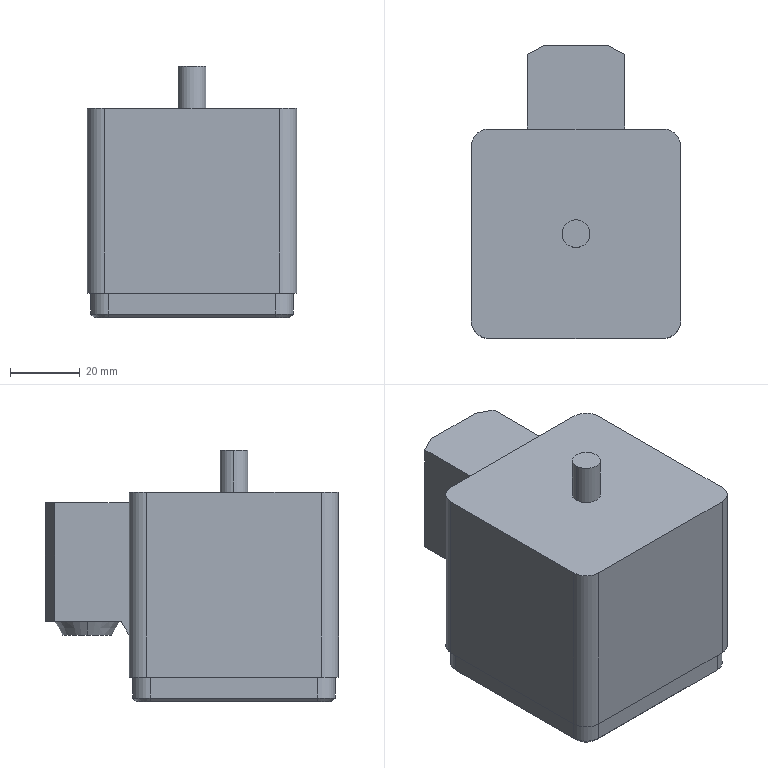Part | SolidWorks | features ICE 5, Fillet 2, Chamfer 1, Extrusion 1 | 1 solid | 41 faces | box 60 x 84 x 72 mm | volume 236948 mm3 | plane 25 | cylinder 10 | cone 6 | commonest cylinder face diameters 10 x8 8 x2
STEP:
#1=CARTESIAN_POINT('',(7.084,42.,19.));
#2=VERTEX_POINT('',#1);
#3=CARTESIAN_POINT('',(-7.084,42.,19.));
#4=VERTEX_POINT('',#3);
#5=CARTESIAN_POINT('',(0.,42.,19.));
#6=DIRECTION('',(0.,0.,-1.));
#7=DIRECTION('',(-1.,0.,0.));
#8=AXIS2_PLACEMENT_3D('',#5,#6,#7);
#9=CIRCLE('',#8,7.084);
#10=EDGE_CURVE('',#2,#4,#9,.T.);
#11=ORIENTED_EDGE('',*,*,#10,.F.);
#12=CARTESIAN_POINT('',(9.393,42.,23.));
#13=VERTEX_POINT('',#12);
#14=CARTESIAN_POINT('',(7.084,42.,19.));
#15=DIRECTION('',(0.5,0.,0.866));
#16=VECTOR('',#15,1000.);
#17=LINE('',#14,#16);
#18=EDGE_CURVE('',#2,#13,#17,.T.);
#19=ORIENTED_EDGE('',*,*,#18,.T.);
#20=CARTESIAN_POINT('',(-9.393,42.,23.));
#21=VERTEX_POINT('',#20);
#22=CARTESIAN_POINT('',(0.,42.,23.));
#23=DIRECTION('',(0.,0.,-1.));
#24=DIRECTION('',(-1.,0.,0.));
#25=AXIS2_PLACEMENT_3D('',#22,#23,#24);
#26=CIRCLE('',#25,9.393);
#27=EDGE_CURVE('',#13,#21,#26,.T.);
#28=ORIENTED_EDGE('',*,*,#27,.T.);
#29=CARTESIAN_POINT('',(-7.084,42.,19.));
#30=DIRECTION('',(-0.5,0.,0.866));
#31=VECTOR('',#30,1000.);
#32=LINE('',#29,#31);
#33=EDGE_CURVE('',#4,#21,#32,.T.);
#34=ORIENTED_EDGE('',*,*,#33,.F.);
#35=EDGE_LOOP('',(#11,#19,#28,#34));
#36=FACE_OUTER_BOUND('',#35,.T.);
#37=CARTESIAN_POINT('',(0.,42.,19.));
#38=DIRECTION('',(0.,0.,1.));
#39=DIRECTION('',(-1.,0.,0.));
#40=AXIS2_PLACEMENT_3D('',#37,#38,#39);
#41=CONICAL_SURFACE('',#40,7.084,0.5236);
#42=ADVANCED_FACE('',(#36),#41,.T.);
#43=CARTESIAN_POINT('',(4.,0.,72.));
#44=VERTEX_POINT('',#43);
#45=CARTESIAN_POINT('',(-4.,0.,72.));
#46=VERTEX_POINT('',#45);
#47=CARTESIAN_POINT('',(0.,0.,72.));
#48=DIRECTION('',(0.,0.,1.));
#49=DIRECTION('',(1.,0.,0.));
#50=AXIS2_PLACEMENT_3D('',#47,#48,#49);
#51=CIRCLE('',#50,4.);
#52=EDGE_CURVE('',#44,#46,#51,.T.);
#53=ORIENTED_EDGE('',*,*,#52,.F.);
#54=CARTESIAN_POINT('',(4.,0.,60.));
#55=VERTEX_POINT('',#54);
#56=CARTESIAN_POINT('',(4.,0.,72.));
#57=DIRECTION('',(0.,0.,-1.));
#58=VECTOR('',#57,1000.);
#59=LINE('',#56,#58);
#60=EDGE_CURVE('',#44,#55,#59,.T.);
#61=ORIENTED_EDGE('',*,*,#60,.T.);
#62=CARTESIAN_POINT('',(-4.,0.,60.));
#63=VERTEX_POINT('',#62);
#64=CARTESIAN_POINT('',(0.,0.,60.));
#65=DIRECTION('',(0.,0.,1.));
#66=DIRECTION('',(-1.,0.,0.));
#67=AXIS2_PLACEMENT_3D('',#64,#65,#66);
#68=CIRCLE('',#67,4.);
#69=EDGE_CURVE('',#55,#63,#68,.T.);
#70=ORIENTED_EDGE('',*,*,#69,.T.);
#71=CARTESIAN_POINT('',(-4.,0.,72.));
#72=DIRECTION('',(0.,0.,-1.));
#73=VECTOR('',#72,1000.);
#74=LINE('',#71,#73);
#75=EDGE_CURVE('',#46,#63,#74,.T.);
#76=ORIENTED_EDGE('',*,*,#75,.F.);
#77=EDGE_LOOP('',(#53,#61,#70,#76));
#78=FACE_OUTER_BOUND('',#77,.T.);
#79=CARTESIAN_POINT('',(0.,0.,72.));
#80=DIRECTION('',(0.,0.,-1.));
#81=DIRECTION('',(-1.,0.,0.));
#82=AXIS2_PLACEMENT_3D('',#79,#80,#81);
#83=CYLINDRICAL_SURFACE('',#82,4.);
#84=ADVANCED_FACE('',(#78),#83,.T.);
#85=CARTESIAN_POINT('',(-9.073,54.,57.));
#86=VERTEX_POINT('',#85);
#87=CARTESIAN_POINT('',(-9.073,54.,23.));
#88=VERTEX_POINT('',#87);
#89=CARTESIAN_POINT('',(-9.073,54.,72.));
#90=DIRECTION('',(0.,0.,-1.));
#91=VECTOR('',#90,1000.);
#92=LINE('',#89,#91);
#93=EDGE_CURVE('',#86,#88,#92,.T.);
#94=ORIENTED_EDGE('',*,*,#93,.F.);
#95=CARTESIAN_POINT('',(9.016,54.,57.));
#96=VERTEX_POINT('',#95);
#97=CARTESIAN_POINT('',(-14.,54.,57.));
#98=DIRECTION('',(1.,0.,0.));
#99=VECTOR('',#98,1000.);
#100=LINE('',#97,#99);
#101=EDGE_CURVE('',#86,#96,#100,.T.);
#102=ORIENTED_EDGE('',*,*,#101,.T.);
#103=CARTESIAN_POINT('',(9.016,54.,23.));
#104=VERTEX_POINT('',#103);
#105=CARTESIAN_POINT('',(9.016,54.,72.));
#106=DIRECTION('',(0.,0.,-1.));
#107=VECTOR('',#106,1000.);
#108=LINE('',#105,#107);
#109=EDGE_CURVE('',#96,#104,#108,.T.);
#110=ORIENTED_EDGE('',*,*,#109,.T.);
#111=CARTESIAN_POINT('',(0.,54.,23.));
#112=DIRECTION('',(-1.,0.,0.));
#113=VECTOR('',#112,1000.);
#114=LINE('',#111,#113);
#115=EDGE_CURVE('',#104,#88,#114,.T.);
#116=ORIENTED_EDGE('',*,*,#115,.T.);
#117=EDGE_LOOP('',(#94,#102,#110,#116));
#118=FACE_OUTER_BOUND('',#117,.T.);
#119=CARTESIAN_POINT('',(0.,54.,0.));
#120=DIRECTION('',(0.,1.,0.));
#121=DIRECTION('',(0.,0.,1.));
#122=AXIS2_PLACEMENT_3D('',#119,#120,#121);
#123=PLANE('',#122);
#124=ADVANCED_FACE('',(#118),#123,.T.);
#125=CARTESIAN_POINT('',(-14.,30.,19.));
#126=VERTEX_POINT('',#125);
#127=CARTESIAN_POINT('',(-14.,30.,57.));
#128=VERTEX_POINT('',#127);
#129=CARTESIAN_POINT('',(-14.,30.,57.));
#130=DIRECTION('',(0.,0.,1.));
#131=VECTOR('',#130,1000.);
#132=LINE('',#129,#131);
#133=EDGE_CURVE('',#126,#128,#132,.T.);
#134=ORIENTED_EDGE('',*,*,#133,.F.);
#135=CARTESIAN_POINT('',(14.,30.,19.));
#136=VERTEX_POINT('',#135);
#137=CARTESIAN_POINT('',(14.,30.,19.));
#138=DIRECTION('',(-1.,0.,0.));
#139=VECTOR('',#138,1000.);
#140=LINE('',#137,#139);
#141=EDGE_CURVE('',#136,#126,#140,.T.);
#142=ORIENTED_EDGE('',*,*,#141,.F.);
#143=CARTESIAN_POINT('',(14.,30.,57.));
#144=VERTEX_POINT('',#143);
#145=CARTESIAN_POINT('',(14.,30.,57.));
#146=DIRECTION('',(0.,0.,-1.));
#147=VECTOR('',#146,1000.);
#148=LINE('',#145,#147);
#149=EDGE_CURVE('',#144,#136,#148,.T.);
#150=ORIENTED_EDGE('',*,*,#149,.F.);
#151=CARTESIAN_POINT('',(-14.,30.,57.));
#152=DIRECTION('',(1.,0.,0.));
#153=VECTOR('',#152,1000.);
#154=LINE('',#151,#153);
#155=EDGE_CURVE('',#128,#144,#154,.T.);
#156=ORIENTED_EDGE('',*,*,#155,.F.);
#157=EDGE_LOOP('',(#134,#142,#150,#156));
#158=FACE_BOUND('',#157,.T.);
#159=CARTESIAN_POINT('',(25.,30.,60.));
#160=VERTEX_POINT('',#159);
#161=CARTESIAN_POINT('',(-25.,30.,60.));
#162=VERTEX_POINT('',#161);
#163=CARTESIAN_POINT('',(-30.,30.,60.));
#164=DIRECTION('',(-1.,0.,0.));
#165=VECTOR('',#164,1000.);
#166=LINE('',#163,#165);
#167=EDGE_CURVE('',#160,#162,#166,.T.);
#168=ORIENTED_EDGE('',*,*,#167,.F.);
#169=CARTESIAN_POINT('',(25.,30.,7.));
#170=VERTEX_POINT('',#169);
#171=CARTESIAN_POINT('',(25.,30.,60.));
#172=DIRECTION('',(0.,0.,-1.));
#173=VECTOR('',#172,1000.);
#174=LINE('',#171,#173);
#175=EDGE_CURVE('',#160,#170,#174,.T.);
#176=ORIENTED_EDGE('',*,*,#175,.T.);
#177=CARTESIAN_POINT('',(-25.,30.,7.));
#178=VERTEX_POINT('',#177);
#179=CARTESIAN_POINT('',(30.,30.,7.));
#180=DIRECTION('',(1.,0.,0.));
#181=VECTOR('',#180,1000.);
#182=LINE('',#179,#181);
#183=EDGE_CURVE('',#178,#170,#182,.T.);
#184=ORIENTED_EDGE('',*,*,#183,.F.);
#185=CARTESIAN_POINT('',(-25.,30.,60.));
#186=DIRECTION('',(0.,0.,1.));
#187=VECTOR('',#186,1000.);
#188=LINE('',#185,#187);
#189=EDGE_CURVE('',#178,#162,#188,.T.);
#190=ORIENTED_EDGE('',*,*,#189,.T.);
#191=EDGE_LOOP('',(#168,#176,#184,#190));
#192=FACE_OUTER_BOUND('',#191,.T.);
#193=CARTESIAN_POINT('',(-30.,30.,60.));
#194=DIRECTION('',(0.,-1.,0.));
#195=DIRECTION('',(0.,0.,-1.));
#196=AXIS2_PLACEMENT_3D('',#193,#194,#195);
#197=PLANE('',#196);
#198=ADVANCED_FACE('',(#158,#192),#197,.F.);
#199=CARTESIAN_POINT('',(30.,-25.,60.));
#200=VERTEX_POINT('',#199);
#201=CARTESIAN_POINT('',(30.,25.,60.));
#202=VERTEX_POINT('',#201);
#203=CARTESIAN_POINT('',(30.,-30.,60.));
#204=DIRECTION('',(0.,1.,0.));
#205=VECTOR('',#204,1000.);
#206=LINE('',#203,#205);
#207=EDGE_CURVE('',#200,#202,#206,.T.);
#208=ORIENTED_EDGE('',*,*,#207,.T.);
#209=CARTESIAN_POINT('',(25.,25.,60.));
#210=DIRECTION('',(0.,0.,1.));
#211=DIRECTION('',(-1.,0.,0.));
#212=AXIS2_PLACEMENT_3D('',#209,#210,#211);
#213=CIRCLE('',#212,5.);
#214=EDGE_CURVE('',#202,#160,#213,.T.);
#215=ORIENTED_EDGE('',*,*,#214,.T.);
#216=ORIENTED_EDGE('',*,*,#167,.T.);
#217=CARTESIAN_POINT('',(-30.,25.,60.));
#218=VERTEX_POINT('',#217);
#219=CARTESIAN_POINT('',(-25.,25.,60.));
#220=DIRECTION('',(0.,0.,1.));
#221=DIRECTION('',(-1.,0.,0.));
#222=AXIS2_PLACEMENT_3D('',#219,#220,#221);
#223=CIRCLE('',#222,5.);
#224=EDGE_CURVE('',#162,#218,#223,.T.);
#225=ORIENTED_EDGE('',*,*,#224,.T.);
#226=CARTESIAN_POINT('',(-30.,-25.,60.));
#227=VERTEX_POINT('',#226);
#228=CARTESIAN_POINT('',(-30.,-30.,60.));
#229=DIRECTION('',(0.,-1.,0.));
#230=VECTOR('',#229,1000.);
#231=LINE('',#228,#230);
#232=EDGE_CURVE('',#218,#227,#231,.T.);
#233=ORIENTED_EDGE('',*,*,#232,.T.);
#234=CARTESIAN_POINT('',(-25.,-30.,60.));
#235=VERTEX_POINT('',#234);
#236=CARTESIAN_POINT('',(-25.,-25.,60.));
#237=DIRECTION('',(0.,0.,1.));
#238=DIRECTION('',(-1.,0.,0.));
#239=AXIS2_PLACEMENT_3D('',#236,#237,#238);
#240=CIRCLE('',#239,5.);
#241=EDGE_CURVE('',#227,#235,#240,.T.);
#242=ORIENTED_EDGE('',*,*,#241,.T.);
#243=CARTESIAN_POINT('',(25.,-30.,60.));
#244=VERTEX_POINT('',#243);
#245=CARTESIAN_POINT('',(-30.,-30.,60.));
#246=DIRECTION('',(1.,0.,0.));
#247=VECTOR('',#246,1000.);
#248=LINE('',#245,#247);
#249=EDGE_CURVE('',#235,#244,#248,.T.);
#250=ORIENTED_EDGE('',*,*,#249,.T.);
#251=CARTESIAN_POINT('',(25.,-25.,60.));
#252=DIRECTION('',(0.,0.,1.));
#253=DIRECTION('',(-1.,0.,0.));
#254=AXIS2_PLACEMENT_3D('',#251,#252,#253);
#255=CIRCLE('',#254,5.);
#256=EDGE_CURVE('',#244,#200,#255,.T.);
#257=ORIENTED_EDGE('',*,*,#256,.T.);
#258=EDGE_LOOP('',(#208,#215,#216,#225,#233,#242,#250,#257));
#259=FACE_OUTER_BOUND('',#258,.T.);
#260=CARTESIAN_POINT('',(0.,0.,60.));
#261=DIRECTION('',(0.,0.,1.));
#262=DIRECTION('',(-1.,0.,0.));
#263=AXIS2_PLACEMENT_3D('',#260,#261,#262);
#264=CIRCLE('',#263,4.);
#265=EDGE_CURVE('',#63,#55,#264,.T.);
#266=ORIENTED_EDGE('',*,*,#265,.F.);
#267=ORIENTED_EDGE('',*,*,#69,.F.);
#268=EDGE_LOOP('',(#266,#267));
#269=FACE_BOUND('',#268,.T.);
#270=CARTESIAN_POINT('',(0.,0.,60.));
#271=DIRECTION('',(0.,0.,-1.));
#272=DIRECTION('',(-1.,0.,0.));
#273=AXIS2_PLACEMENT_3D('',#270,#271,#272);
#274=PLANE('',#273);
#275=ADVANCED_FACE('',(#259,#269),#274,.F.);
#276=CARTESIAN_POINT('',(30.,25.,7.));
#277=VERTEX_POINT('',#276);
#278=CARTESIAN_POINT('',(30.,-25.,7.));
#279=VERTEX_POINT('',#278);
#280=CARTESIAN_POINT('',(30.,-30.,7.));
#281=DIRECTION('',(0.,-1.,0.));
#282=VECTOR('',#281,1000.);
#283=LINE('',#280,#282);
#284=EDGE_CURVE('',#277,#279,#283,.T.);
#285=ORIENTED_EDGE('',*,*,#284,.F.);
#286=CARTESIAN_POINT('',(30.,25.,60.));
#287=DIRECTION('',(0.,0.,1.));
#288=VECTOR('',#287,1000.);
#289=LINE('',#286,#288);
#290=EDGE_CURVE('',#277,#202,#289,.T.);
#291=ORIENTED_EDGE('',*,*,#290,.T.);
#292=ORIENTED_EDGE('',*,*,#207,.F.);
#293=CARTESIAN_POINT('',(30.,-25.,60.));
#294=DIRECTION('',(0.,0.,-1.));
#295=VECTOR('',#294,1000.);
#296=LINE('',#293,#295);
#297=EDGE_CURVE('',#200,#279,#296,.T.);
#298=ORIENTED_EDGE('',*,*,#297,.T.);
#299=EDGE_LOOP('',(#285,#291,#292,#298));
#300=FACE_OUTER_BOUND('',#299,.T.);
#301=CARTESIAN_POINT('',(30.,-30.,60.));
#302=DIRECTION('',(-1.,0.,0.));
#303=DIRECTION('',(0.,0.,1.));
#304=AXIS2_PLACEMENT_3D('',#301,#302,#303);
#305=PLANE('',#304);
#306=ADVANCED_FACE('',(#300),#305,.F.);
#307=CARTESIAN_POINT('',(-30.,-25.,7.));
#308=VERTEX_POINT('',#307);
#309=CARTESIAN_POINT('',(-30.,25.,7.));
#310=VERTEX_POINT('',#309);
#311=CARTESIAN_POINT('',(-30.,-30.,7.));
#312=DIRECTION('',(0.,1.,0.));
#313=VECTOR('',#312,1000.);
#314=LINE('',#311,#313);
#315=EDGE_CURVE('',#308,#310,#314,.T.);
#316=ORIENTED_EDGE('',*,*,#315,.F.);
#317=CARTESIAN_POINT('',(-30.,-25.,60.));
#318=DIRECTION('',(0.,0.,1.));
#319=VECTOR('',#318,1000.);
#320=LINE('',#317,#319);
#321=EDGE_CURVE('',#308,#227,#320,.T.);
#322=ORIENTED_EDGE('',*,*,#321,.T.);
#323=ORIENTED_EDGE('',*,*,#232,.F.);
#324=CARTESIAN_POINT('',(-30.,25.,60.));
#325=DIRECTION('',(0.,0.,-1.));
#326=VECTOR('',#325,1000.);
#327=LINE('',#324,#326);
#328=EDGE_CURVE('',#218,#310,#327,.T.);
#329=ORIENTED_EDGE('',*,*,#328,.T.);
#330=EDGE_LOOP('',(#316,#322,#323,#329));
#331=FACE_OUTER_BOUND('',#330,.T.);
#332=CARTESIAN_POINT('',(-30.,-30.,60.));
#333=DIRECTION('',(1.,0.,0.));
#334=DIRECTION('',(0.,0.,-1.));
#335=AXIS2_PLACEMENT_3D('',#332,#333,#334);
#336=PLANE('',#335);
#337=ADVANCED_FACE('',(#331),#336,.F.);
#338=CARTESIAN_POINT('',(25.,-30.,7.));
#339=VERTEX_POINT('',#338);
#340=CARTESIAN_POINT('',(-25.,-30.,7.));
#341=VERTEX_POINT('',#340);
#342=CARTESIAN_POINT('',(30.,-30.,7.));
#343=DIRECTION('',(-1.,0.,0.));
#344=VECTOR('',#343,1000.);
#345=LINE('',#342,#344);
#346=EDGE_CURVE('',#339,#341,#345,.T.);
#347=ORIENTED_EDGE('',*,*,#346,.F.);
#348=CARTESIAN_POINT('',(25.,-30.,60.));
#349=DIRECTION('',(0.,0.,1.));
#350=VECTOR('',#349,1000.);
#351=LINE('',#348,#350);
#352=EDGE_CURVE('',#339,#244,#351,.T.);
#353=ORIENTED_EDGE('',*,*,#352,.T.);
#354=ORIENTED_EDGE('',*,*,#249,.F.);
#355=CARTESIAN_POINT('',(-25.,-30.,60.));
#356=DIRECTION('',(0.,0.,-1.));
#357=VECTOR('',#356,1000.);
#358=LINE('',#355,#357);
#359=EDGE_CURVE('',#235,#341,#358,.T.);
#360=ORIENTED_EDGE('',*,*,#359,.T.);
#361=EDGE_LOOP('',(#347,#353,#354,#360));
#362=FACE_OUTER_BOUND('',#361,.T.);
#363=CARTESIAN_POINT('',(-30.,-30.,60.));
#364=DIRECTION('',(0.,1.,0.));
#365=DIRECTION('',(0.,0.,1.));
#366=AXIS2_PLACEMENT_3D('',#363,#364,#365);
#367=PLANE('',#366);
#368=ADVANCED_FACE('',(#362),#367,.F.);
#369=ORIENTED_EDGE('',*,*,#60,.F.);
#370=CARTESIAN_POINT('',(0.,0.,72.));
#371=DIRECTION('',(0.,0.,1.));
#372=DIRECTION('',(1.,0.,0.));
#373=AXIS2_PLACEMENT_3D('',#370,#371,#372);
#374=CIRCLE('',#373,4.);
#375=EDGE_CURVE('',#46,#44,#374,.T.);
#376=ORIENTED_EDGE('',*,*,#375,.F.);
#377=ORIENTED_EDGE('',*,*,#75,.T.);
#378=ORIENTED_EDGE('',*,*,#265,.T.);
#379=EDGE_LOOP('',(#369,#376,#377,#378));
#380=FACE_OUTER_BOUND('',#379,.T.);
#381=CARTESIAN_POINT('',(0.,0.,72.));
#382=DIRECTION('',(0.,0.,-1.));
#383=DIRECTION('',(-1.,0.,0.));
#384=AXIS2_PLACEMENT_3D('',#381,#382,#383);
#385=CYLINDRICAL_SURFACE('',#384,4.);
#386=ADVANCED_FACE('',(#380),#385,.T.);
#387=ORIENTED_EDGE('',*,*,#375,.T.);
#388=ORIENTED_EDGE('',*,*,#52,.T.);
#389=EDGE_LOOP('',(#387,#388));
#390=FACE_OUTER_BOUND('',#389,.T.);
#391=CARTESIAN_POINT('',(0.,0.,72.));
#392=DIRECTION('',(0.,0.,1.));
#393=DIRECTION('',(1.,0.,0.));
#394=AXIS2_PLACEMENT_3D('',#391,#392,#393);
#395=PLANE('',#394);
#396=ADVANCED_FACE('',(#390),#395,.T.);
#397=CARTESIAN_POINT('',(-29.,-24.,7.));
#398=VERTEX_POINT('',#397);
#399=CARTESIAN_POINT('',(-29.,24.,7.));
#400=VERTEX_POINT('',#399);
#401=CARTESIAN_POINT('',(-29.,-29.,7.));
#402=DIRECTION('',(0.,1.,0.));
#403=VECTOR('',#402,1000.);
#404=LINE('',#401,#403);
#405=EDGE_CURVE('',#398,#400,#404,.T.);
#406=ORIENTED_EDGE('',*,*,#405,.F.);
#407=CARTESIAN_POINT('',(-24.,-29.,7.));
#408=VERTEX_POINT('',#407);
#409=CARTESIAN_POINT('',(-24.,-24.,7.));
#410=DIRECTION('',(0.,0.,1.));
#411=DIRECTION('',(1.,0.,0.));
#412=AXIS2_PLACEMENT_3D('',#409,#410,#411);
#413=CIRCLE('',#412,5.);
#414=EDGE_CURVE('',#398,#408,#413,.T.);
#415=ORIENTED_EDGE('',*,*,#414,.T.);
#416=CARTESIAN_POINT('',(24.,-29.,7.));
#417=VERTEX_POINT('',#416);
#418=CARTESIAN_POINT('',(29.,-29.,7.));
#419=DIRECTION('',(-1.,0.,0.));
#420=VECTOR('',#419,1000.);
#421=LINE('',#418,#420);
#422=EDGE_CURVE('',#417,#408,#421,.T.);
#423=ORIENTED_EDGE('',*,*,#422,.F.);
#424=CARTESIAN_POINT('',(29.,-24.,7.));
#425=VERTEX_POINT('',#424);
#426=CARTESIAN_POINT('',(24.,-24.,7.));
#427=DIRECTION('',(0.,0.,1.));
#428=DIRECTION('',(1.,0.,0.));
#429=AXIS2_PLACEMENT_3D('',#426,#427,#428);
#430=CIRCLE('',#429,5.);
#431=EDGE_CURVE('',#417,#425,#430,.T.);
#432=ORIENTED_EDGE('',*,*,#431,.T.);
#433=CARTESIAN_POINT('',(29.,24.,7.));
#434=VERTEX_POINT('',#433);
#435=CARTESIAN_POINT('',(29.,-29.,7.));
#436=DIRECTION('',(0.,-1.,0.));
#437=VECTOR('',#436,1000.);
#438=LINE('',#435,#437);
#439=EDGE_CURVE('',#434,#425,#438,.T.);
#440=ORIENTED_EDGE('',*,*,#439,.F.);
#441=CARTESIAN_POINT('',(24.,29.,7.));
#442=VERTEX_POINT('',#441);
#443=CARTESIAN_POINT('',(24.,24.,7.));
#444=DIRECTION('',(0.,0.,1.));
#445=DIRECTION('',(1.,0.,0.));
#446=AXIS2_PLACEMENT_3D('',#443,#444,#445);
#447=CIRCLE('',#446,5.);
#448=EDGE_CURVE('',#434,#442,#447,.T.);
#449=ORIENTED_EDGE('',*,*,#448,.T.);
#450=CARTESIAN_POINT('',(-24.,29.,7.));
#451=VERTEX_POINT('',#450);
#452=CARTESIAN_POINT('',(29.,29.,7.));
#453=DIRECTION('',(1.,0.,0.));
#454=VECTOR('',#453,1000.);
#455=LINE('',#452,#454);
#456=EDGE_CURVE('',#451,#442,#455,.T.);
#457=ORIENTED_EDGE('',*,*,#456,.F.);
#458=CARTESIAN_POINT('',(-24.,24.,7.));
#459=DIRECTION('',(0.,0.,1.));
#460=DIRECTION('',(1.,0.,0.));
#461=AXIS2_PLACEMENT_3D('',#458,#459,#460);
#462=CIRCLE('',#461,5.);
#463=EDGE_CURVE('',#451,#400,#462,.T.);
#464=ORIENTED_EDGE('',*,*,#463,.T.);
#465=EDGE_LOOP('',(#406,#415,#423,#432,#440,#449,#457,#464));
#466=FACE_BOUND('',#465,.T.);
#467=ORIENTED_EDGE('',*,*,#183,.T.);
#468=CARTESIAN_POINT('',(25.,25.,7.));
#469=DIRECTION('',(0.,0.,-1.));
#470=DIRECTION('',(1.,0.,0.));
#471=AXIS2_PLACEMENT_3D('',#468,#469,#470);
#472=CIRCLE('',#471,5.);
#473=EDGE_CURVE('',#170,#277,#472,.T.);
#474=ORIENTED_EDGE('',*,*,#473,.T.);
#475=ORIENTED_EDGE('',*,*,#284,.T.);
#476=CARTESIAN_POINT('',(25.,-25.,7.));
#477=DIRECTION('',(0.,0.,-1.));
#478=DIRECTION('',(1.,0.,0.));
#479=AXIS2_PLACEMENT_3D('',#476,#477,#478);
#480=CIRCLE('',#479,5.);
#481=EDGE_CURVE('',#279,#339,#480,.T.);
#482=ORIENTED_EDGE('',*,*,#481,.T.);
#483=ORIENTED_EDGE('',*,*,#346,.T.);
#484=CARTESIAN_POINT('',(-25.,-25.,7.));
#485=DIRECTION('',(0.,0.,-1.));
#486=DIRECTION('',(1.,0.,0.));
#487=AXIS2_PLACEMENT_3D('',#484,#485,#486);
#488=CIRCLE('',#487,5.);
#489=EDGE_CURVE('',#341,#308,#488,.T.);
#490=ORIENTED_EDGE('',*,*,#489,.T.);
#491=ORIENTED_EDGE('',*,*,#315,.T.);
#492=CARTESIAN_POINT('',(-25.,25.,7.));
#493=DIRECTION('',(0.,0.,-1.));
#494=DIRECTION('',(1.,0.,0.));
#495=AXIS2_PLACEMENT_3D('',#492,#493,#494);
#496=CIRCLE('',#495,5.);
#497=EDGE_CURVE('',#310,#178,#496,.T.);
#498=ORIENTED_EDGE('',*,*,#497,.T.);
#499=EDGE_LOOP('',(#467,#474,#475,#482,#483,#490,#491,#498));
#500=FACE_OUTER_BOUND('',#499,.T.);
#501=CARTESIAN_POINT('',(0.,0.,7.));
#502=DIRECTION('',(0.,0.,1.));
#503=DIRECTION('',(1.,0.,0.));
#504=AXIS2_PLACEMENT_3D('',#501,#502,#503);
#505=PLANE('',#504);
#506=ADVANCED_FACE('',(#466,#500),#505,.F.);
#507=CARTESIAN_POINT('',(-29.,24.,1.));
#508=VERTEX_POINT('',#507);
#509=CARTESIAN_POINT('',(-29.,24.,7.));
#510=DIRECTION('',(0.,0.,-1.));
#511=VECTOR('',#510,1000.);
#512=LINE('',#509,#511);
#513=EDGE_CURVE('',#400,#508,#512,.T.);
#514=ORIENTED_EDGE('',*,*,#513,.T.);
#515=CARTESIAN_POINT('',(-29.,-24.,1.));
#516=VERTEX_POINT('',#515);
#517=CARTESIAN_POINT('',(-29.,-29.,1.));
#518=DIRECTION('',(0.,-1.,0.));
#519=VECTOR('',#518,1000.);
#520=LINE('',#517,#519);
#521=EDGE_CURVE('',#508,#516,#520,.T.);
#522=ORIENTED_EDGE('',*,*,#521,.T.);
#523=CARTESIAN_POINT('',(-29.,-24.,7.));
#524=DIRECTION('',(0.,0.,1.));
#525=VECTOR('',#524,1000.);
#526=LINE('',#523,#525);
#527=EDGE_CURVE('',#516,#398,#526,.T.);
#528=ORIENTED_EDGE('',*,*,#527,.T.);
#529=ORIENTED_EDGE('',*,*,#405,.T.);
#530=EDGE_LOOP('',(#514,#522,#528,#529));
#531=FACE_OUTER_BOUND('',#530,.T.);
#532=CARTESIAN_POINT('',(-29.,-29.,7.));
#533=DIRECTION('',(-1.,0.,0.));
#534=DIRECTION('',(0.,0.,1.));
#535=AXIS2_PLACEMENT_3D('',#532,#533,#534);
#536=PLANE('',#535);
#537=ADVANCED_FACE('',(#531),#536,.T.);
#538=CARTESIAN_POINT('',(-24.,-29.,1.));
#539=VERTEX_POINT('',#538);
#540=CARTESIAN_POINT('',(-24.,-29.,7.));
#541=DIRECTION('',(0.,0.,-1.));
#542=VECTOR('',#541,1000.);
#543=LINE('',#540,#542);
#544=EDGE_CURVE('',#408,#539,#543,.T.);
#545=ORIENTED_EDGE('',*,*,#544,.T.);
#546=CARTESIAN_POINT('',(24.,-29.,1.));
#547=VERTEX_POINT('',#546);
#548=CARTESIAN_POINT('',(29.,-29.,1.));
#549=DIRECTION('',(1.,0.,0.));
#550=VECTOR('',#549,1000.);
#551=LINE('',#548,#550);
#552=EDGE_CURVE('',#539,#547,#551,.T.);
#553=ORIENTED_EDGE('',*,*,#552,.T.);
#554=CARTESIAN_POINT('',(24.,-29.,7.));
#555=DIRECTION('',(0.,0.,1.));
#556=VECTOR('',#555,1000.);
#557=LINE('',#554,#556);
#558=EDGE_CURVE('',#547,#417,#557,.T.);
#559=ORIENTED_EDGE('',*,*,#558,.T.);
#560=ORIENTED_EDGE('',*,*,#422,.T.);
#561=EDGE_LOOP('',(#545,#553,#559,#560));
#562=FACE_OUTER_BOUND('',#561,.T.);
#563=CARTESIAN_POINT('',(29.,-29.,7.));
#564=DIRECTION('',(0.,-1.,0.));
#565=DIRECTION('',(0.,0.,-1.));
#566=AXIS2_PLACEMENT_3D('',#563,#564,#565);
#567=PLANE('',#566);
#568=ADVANCED_FACE('',(#562),#567,.T.);
#569=CARTESIAN_POINT('',(29.,-24.,1.));
#570=VERTEX_POINT('',#569);
#571=CARTESIAN_POINT('',(29.,-24.,7.));
#572=DIRECTION('',(0.,0.,-1.));
#573=VECTOR('',#572,1000.);
#574=LINE('',#571,#573);
#575=EDGE_CURVE('',#425,#570,#574,.T.);
#576=ORIENTED_EDGE('',*,*,#575,.T.);
#577=CARTESIAN_POINT('',(29.,24.,1.));
#578=VERTEX_POINT('',#577);
#579=CARTESIAN_POINT('',(29.,-29.,1.));
#580=DIRECTION('',(0.,1.,0.));
#581=VECTOR('',#580,1000.);
#582=LINE('',#579,#581);
#583=EDGE_CURVE('',#570,#578,#582,.T.);
#584=ORIENTED_EDGE('',*,*,#583,.T.);
#585=CARTESIAN_POINT('',(29.,24.,7.));
#586=DIRECTION('',(0.,0.,1.));
#587=VECTOR('',#586,1000.);
#588=LINE('',#585,#587);
#589=EDGE_CURVE('',#578,#434,#588,.T.);
#590=ORIENTED_EDGE('',*,*,#589,.T.);
#591=ORIENTED_EDGE('',*,*,#439,.T.);
#592=EDGE_LOOP('',(#576,#584,#590,#591));
#593=FACE_OUTER_BOUND('',#592,.T.);
#594=CARTESIAN_POINT('',(29.,-29.,7.));
#595=DIRECTION('',(1.,0.,0.));
#596=DIRECTION('',(0.,0.,-1.));
#597=AXIS2_PLACEMENT_3D('',#594,#595,#596);
#598=PLANE('',#597);
#599=ADVANCED_FACE('',(#593),#598,.T.);
#600=CARTESIAN_POINT('',(24.,29.,1.));
#601=VERTEX_POINT('',#600);
#602=CARTESIAN_POINT('',(24.,29.,7.));
#603=DIRECTION('',(0.,0.,-1.));
#604=VECTOR('',#603,1000.);
#605=LINE('',#602,#604);
#606=EDGE_CURVE('',#442,#601,#605,.T.);
#607=ORIENTED_EDGE('',*,*,#606,.T.);
#608=CARTESIAN_POINT('',(-24.,29.,1.));
#609=VERTEX_POINT('',#608);
#610=CARTESIAN_POINT('',(29.,29.,1.));
#611=DIRECTION('',(-1.,0.,0.));
#612=VECTOR('',#611,1000.);
#613=LINE('',#610,#612);
#614=EDGE_CURVE('',#601,#609,#613,.T.);
#615=ORIENTED_EDGE('',*,*,#614,.T.);
#616=CARTESIAN_POINT('',(-24.,29.,7.));
#617=DIRECTION('',(0.,0.,1.));
#618=VECTOR('',#617,1000.);
#619=LINE('',#616,#618);
#620=EDGE_CURVE('',#609,#451,#619,.T.);
#621=ORIENTED_EDGE('',*,*,#620,.T.);
#622=ORIENTED_EDGE('',*,*,#456,.T.);
#623=EDGE_LOOP('',(#607,#615,#621,#622));
#624=FACE_OUTER_BOUND('',#623,.T.);
#625=CARTESIAN_POINT('',(29.,29.,7.));
#626=DIRECTION('',(0.,1.,0.));
#627=DIRECTION('',(0.,0.,1.));
#628=AXIS2_PLACEMENT_3D('',#625,#626,#627);
#629=PLANE('',#628);
#630=ADVANCED_FACE('',(#624),#629,.T.);
#631=CARTESIAN_POINT('',(-28.,-24.,0.));
#632=VERTEX_POINT('',#631);
#633=CARTESIAN_POINT('',(-28.,24.,0.));
#634=VERTEX_POINT('',#633);
#635=CARTESIAN_POINT('',(-28.,0.,0.));
#636=DIRECTION('',(0.,1.,0.));
#637=VECTOR('',#636,1000.);
#638=LINE('',#635,#637);
#639=EDGE_CURVE('',#632,#634,#638,.T.);
#640=ORIENTED_EDGE('',*,*,#639,.T.);
#641=CARTESIAN_POINT('',(-24.,28.,0.));
#642=VERTEX_POINT('',#641);
#643=CARTESIAN_POINT('',(-24.,24.,0.));
#644=DIRECTION('',(0.,0.,-1.));
#645=DIRECTION('',(-1.,0.,0.));
#646=AXIS2_PLACEMENT_3D('',#643,#644,#645);
#647=CIRCLE('',#646,4.);
#648=EDGE_CURVE('',#634,#642,#647,.T.);
#649=ORIENTED_EDGE('',*,*,#648,.T.);
#650=CARTESIAN_POINT('',(24.,28.,0.));
#651=VERTEX_POINT('',#650);
#652=CARTESIAN_POINT('',(0.,28.,0.));
#653=DIRECTION('',(1.,0.,0.));
#654=VECTOR('',#653,1000.);
#655=LINE('',#652,#654);
#656=EDGE_CURVE('',#642,#651,#655,.T.);
#657=ORIENTED_EDGE('',*,*,#656,.T.);
#658=CARTESIAN_POINT('',(28.,24.,0.));
#659=VERTEX_POINT('',#658);
#660=CARTESIAN_POINT('',(24.,24.,0.));
#661=DIRECTION('',(0.,0.,-1.));
#662=DIRECTION('',(-1.,0.,0.));
#663=AXIS2_PLACEMENT_3D('',#660,#661,#662);
#664=CIRCLE('',#663,4.);
#665=EDGE_CURVE('',#651,#659,#664,.T.);
#666=ORIENTED_EDGE('',*,*,#665,.T.);
#667=CARTESIAN_POINT('',(28.,-24.,0.));
#668=VERTEX_POINT('',#667);
#669=CARTESIAN_POINT('',(28.,0.,0.));
#670=DIRECTION('',(0.,-1.,0.));
#671=VECTOR('',#670,1000.);
#672=LINE('',#669,#671);
#673=EDGE_CURVE('',#659,#668,#672,.T.);
#674=ORIENTED_EDGE('',*,*,#673,.T.);
#675=CARTESIAN_POINT('',(24.,-28.,0.));
#676=VERTEX_POINT('',#675);
#677=CARTESIAN_POINT('',(24.,-24.,0.));
#678=DIRECTION('',(0.,0.,-1.));
#679=DIRECTION('',(-1.,0.,0.));
#680=AXIS2_PLACEMENT_3D('',#677,#678,#679);
#681=CIRCLE('',#680,4.);
#682=EDGE_CURVE('',#668,#676,#681,.T.);
#683=ORIENTED_EDGE('',*,*,#682,.T.);
#684=CARTESIAN_POINT('',(-24.,-28.,0.));
#685=VERTEX_POINT('',#684);
#686=CARTESIAN_POINT('',(0.,-28.,0.));
#687=DIRECTION('',(-1.,0.,0.));
#688=VECTOR('',#687,1000.);
#689=LINE('',#686,#688);
#690=EDGE_CURVE('',#676,#685,#689,.T.);
#691=ORIENTED_EDGE('',*,*,#690,.T.);
#692=CARTESIAN_POINT('',(-24.,-24.,0.));
#693=DIRECTION('',(0.,0.,-1.));
#694=DIRECTION('',(-1.,0.,0.));
#695=AXIS2_PLACEMENT_3D('',#692,#693,#694);
#696=CIRCLE('',#695,4.);
#697=EDGE_CURVE('',#685,#632,#696,.T.);
#698=ORIENTED_EDGE('',*,*,#697,.T.);
#699=EDGE_LOOP('',(#640,#649,#657,#666,#674,#683,#691,#698));
#700=FACE_OUTER_BOUND('',#699,.T.);
#701=CARTESIAN_POINT('',(0.,0.,0.));
#702=DIRECTION('',(0.,0.,-1.));
#703=DIRECTION('',(-1.,0.,0.));
#704=AXIS2_PLACEMENT_3D('',#701,#702,#703);
#705=PLANE('',#704);
#706=ADVANCED_FACE('',(#700),#705,.T.);
#707=ORIENTED_EDGE('',*,*,#620,.F.);
#708=CARTESIAN_POINT('',(-24.,24.,1.));
#709=DIRECTION('',(0.,0.,1.));
#710=DIRECTION('',(-1.,0.,0.));
#711=AXIS2_PLACEMENT_3D('',#708,#709,#710);
#712=CIRCLE('',#711,5.);
#713=EDGE_CURVE('',#609,#508,#712,.T.);
#714=ORIENTED_EDGE('',*,*,#713,.T.);
#715=ORIENTED_EDGE('',*,*,#513,.F.);
#716=ORIENTED_EDGE('',*,*,#463,.F.);
#717=EDGE_LOOP('',(#707,#714,#715,#716));
#718=FACE_OUTER_BOUND('',#717,.T.);
#719=CARTESIAN_POINT('',(-24.,24.,7.));
#720=DIRECTION('',(0.,0.,-1.));
#721=DIRECTION('',(-1.,0.,0.));
#722=AXIS2_PLACEMENT_3D('',#719,#720,#721);
#723=CYLINDRICAL_SURFACE('',#722,5.);
#724=ADVANCED_FACE('',(#718),#723,.T.);
#725=ORIENTED_EDGE('',*,*,#527,.F.);
#726=CARTESIAN_POINT('',(-24.,-24.,1.));
#727=DIRECTION('',(0.,0.,1.));
#728=DIRECTION('',(-1.,0.,0.));
#729=AXIS2_PLACEMENT_3D('',#726,#727,#728);
#730=CIRCLE('',#729,5.);
#731=EDGE_CURVE('',#516,#539,#730,.T.);
#732=ORIENTED_EDGE('',*,*,#731,.T.);
#733=ORIENTED_EDGE('',*,*,#544,.F.);
#734=ORIENTED_EDGE('',*,*,#414,.F.);
#735=EDGE_LOOP('',(#725,#732,#733,#734));
#736=FACE_OUTER_BOUND('',#735,.T.);
#737=CARTESIAN_POINT('',(-24.,-24.,7.));
#738=DIRECTION('',(0.,0.,-1.));
#739=DIRECTION('',(-1.,0.,0.));
#740=AXIS2_PLACEMENT_3D('',#737,#738,#739);
#741=CYLINDRICAL_SURFACE('',#740,5.);
#742=ADVANCED_FACE('',(#736),#741,.T.);
#743=ORIENTED_EDGE('',*,*,#558,.F.);
#744=CARTESIAN_POINT('',(24.,-24.,1.));
#745=DIRECTION('',(0.,0.,1.));
#746=DIRECTION('',(-1.,0.,0.));
#747=AXIS2_PLACEMENT_3D('',#744,#745,#746);
#748=CIRCLE('',#747,5.);
#749=EDGE_CURVE('',#547,#570,#748,.T.);
#750=ORIENTED_EDGE('',*,*,#749,.T.);
#751=ORIENTED_EDGE('',*,*,#575,.F.);
#752=ORIENTED_EDGE('',*,*,#431,.F.);
#753=EDGE_LOOP('',(#743,#750,#751,#752));
#754=FACE_OUTER_BOUND('',#753,.T.);
#755=CARTESIAN_POINT('',(24.,-24.,7.));
#756=DIRECTION('',(0.,0.,-1.));
#757=DIRECTION('',(-1.,0.,0.));
#758=AXIS2_PLACEMENT_3D('',#755,#756,#757);
#759=CYLINDRICAL_SURFACE('',#758,5.);
#760=ADVANCED_FACE('',(#754),#759,.T.);
#761=ORIENTED_EDGE('',*,*,#589,.F.);
#762=CARTESIAN_POINT('',(24.,24.,1.));
#763=DIRECTION('',(0.,0.,1.));
#764=DIRECTION('',(-1.,0.,0.));
#765=AXIS2_PLACEMENT_3D('',#762,#763,#764);
#766=CIRCLE('',#765,5.);
#767=EDGE_CURVE('',#578,#601,#766,.T.);
#768=ORIENTED_EDGE('',*,*,#767,.T.);
#769=ORIENTED_EDGE('',*,*,#606,.F.);
#770=ORIENTED_EDGE('',*,*,#448,.F.);
#771=EDGE_LOOP('',(#761,#768,#769,#770));
#772=FACE_OUTER_BOUND('',#771,.T.);
#773=CARTESIAN_POINT('',(24.,24.,7.));
#774=DIRECTION('',(0.,0.,-1.));
#775=DIRECTION('',(-1.,0.,0.));
#776=AXIS2_PLACEMENT_3D('',#773,#774,#775);
#777=CYLINDRICAL_SURFACE('',#776,5.);
#778=ADVANCED_FACE('',(#772),#777,.T.);
#779=CARTESIAN_POINT('',(29.,-24.,1.));
#780=DIRECTION('',(-0.7071,0.,-0.7071));
#781=VECTOR('',#780,1000.);
#782=LINE('',#779,#781);
#783=EDGE_CURVE('',#570,#668,#782,.T.);
#784=ORIENTED_EDGE('',*,*,#783,.F.);
#785=ORIENTED_EDGE('',*,*,#749,.F.);
#786=CARTESIAN_POINT('',(24.,-28.,0.));
#787=DIRECTION('',(0.,-0.7071,0.7071));
#788=VECTOR('',#787,1000.);
#789=LINE('',#786,#788);
#790=EDGE_CURVE('',#676,#547,#789,.T.);
#791=ORIENTED_EDGE('',*,*,#790,.F.);
#792=ORIENTED_EDGE('',*,*,#682,.F.);
#793=EDGE_LOOP('',(#784,#785,#791,#792));
#794=FACE_OUTER_BOUND('',#793,.T.);
#795=CARTESIAN_POINT('',(24.,-24.,0.));
#796=DIRECTION('',(0.,0.,1.));
#797=DIRECTION('',(1.,0.,0.));
#798=AXIS2_PLACEMENT_3D('',#795,#796,#797);
#799=CONICAL_SURFACE('',#798,4.,0.7854);
#800=ADVANCED_FACE('',(#794),#799,.T.);
#801=ORIENTED_EDGE('',*,*,#790,.T.);
#802=ORIENTED_EDGE('',*,*,#552,.F.);
#803=CARTESIAN_POINT('',(-24.,-28.,0.));
#804=DIRECTION('',(0.,-0.7071,0.7071));
#805=VECTOR('',#804,1000.);
#806=LINE('',#803,#805);
#807=EDGE_CURVE('',#685,#539,#806,.T.);
#808=ORIENTED_EDGE('',*,*,#807,.F.);
#809=ORIENTED_EDGE('',*,*,#690,.F.);
#810=EDGE_LOOP('',(#801,#802,#808,#809));
#811=FACE_OUTER_BOUND('',#810,.T.);
#812=CARTESIAN_POINT('',(0.,-28.,0.));
#813=DIRECTION('',(0.,0.7071,0.7071));
#814=DIRECTION('',(-1.,0.,0.));
#815=AXIS2_PLACEMENT_3D('',#812,#813,#814);
#816=PLANE('',#815);
#817=ADVANCED_FACE('',(#811),#816,.F.);
#818=ORIENTED_EDGE('',*,*,#783,.T.);
#819=ORIENTED_EDGE('',*,*,#673,.F.);
#820=CARTESIAN_POINT('',(29.,24.,1.));
#821=DIRECTION('',(-0.7071,0.,-0.7071));
#822=VECTOR('',#821,1000.);
#823=LINE('',#820,#822);
#824=EDGE_CURVE('',#578,#659,#823,.T.);
#825=ORIENTED_EDGE('',*,*,#824,.F.);
#826=ORIENTED_EDGE('',*,*,#583,.F.);
#827=EDGE_LOOP('',(#818,#819,#825,#826));
#828=FACE_OUTER_BOUND('',#827,.T.);
#829=CARTESIAN_POINT('',(28.,0.,0.));
#830=DIRECTION('',(-0.7071,0.,0.7071));
#831=DIRECTION('',(0.,-1.,0.));
#832=AXIS2_PLACEMENT_3D('',#829,#830,#831);
#833=PLANE('',#832);
#834=ADVANCED_FACE('',(#828),#833,.F.);
#835=ORIENTED_EDGE('',*,*,#807,.T.);
#836=ORIENTED_EDGE('',*,*,#731,.F.);
#837=CARTESIAN_POINT('',(-28.,-24.,0.));
#838=DIRECTION('',(-0.7071,0.,0.7071));
#839=VECTOR('',#838,1000.);
#840=LINE('',#837,#839);
#841=EDGE_CURVE('',#632,#516,#840,.T.);
#842=ORIENTED_EDGE('',*,*,#841,.F.);
#843=ORIENTED_EDGE('',*,*,#697,.F.);
#844=EDGE_LOOP('',(#835,#836,#842,#843));
#845=FACE_OUTER_BOUND('',#844,.T.);
#846=CARTESIAN_POINT('',(-24.,-24.,0.));
#847=DIRECTION('',(0.,0.,1.));
#848=DIRECTION('',(1.,0.,0.));
#849=AXIS2_PLACEMENT_3D('',#846,#847,#848);
#850=CONICAL_SURFACE('',#849,4.,0.7854);
#851=ADVANCED_FACE('',(#845),#850,.T.);
#852=ORIENTED_EDGE('',*,*,#824,.T.);
#853=ORIENTED_EDGE('',*,*,#665,.F.);
#854=CARTESIAN_POINT('',(24.,29.,1.));
#855=DIRECTION('',(0.,-0.7071,-0.7071));
#856=VECTOR('',#855,1000.);
#857=LINE('',#854,#856);
#858=EDGE_CURVE('',#601,#651,#857,.T.);
#859=ORIENTED_EDGE('',*,*,#858,.F.);
#860=ORIENTED_EDGE('',*,*,#767,.F.);
#861=EDGE_LOOP('',(#852,#853,#859,#860));
#862=FACE_OUTER_BOUND('',#861,.T.);
#863=CARTESIAN_POINT('',(24.,24.,0.));
#864=DIRECTION('',(0.,0.,1.));
#865=DIRECTION('',(1.,0.,0.));
#866=AXIS2_PLACEMENT_3D('',#863,#864,#865);
#867=CONICAL_SURFACE('',#866,4.,0.7854);
#868=ADVANCED_FACE('',(#862),#867,.T.);
#869=ORIENTED_EDGE('',*,*,#841,.T.);
#870=ORIENTED_EDGE('',*,*,#521,.F.);
#871=CARTESIAN_POINT('',(-28.,24.,0.));
#872=DIRECTION('',(-0.7071,0.,0.7071));
#873=VECTOR('',#872,1000.);
#874=LINE('',#871,#873);
#875=EDGE_CURVE('',#634,#508,#874,.T.);
#876=ORIENTED_EDGE('',*,*,#875,.F.);
#877=ORIENTED_EDGE('',*,*,#639,.F.);
#878=EDGE_LOOP('',(#869,#870,#876,#877));
#879=FACE_OUTER_BOUND('',#878,.T.);
#880=CARTESIAN_POINT('',(-28.,0.,0.));
#881=DIRECTION('',(0.7071,0.,0.7071));
#882=DIRECTION('',(0.,1.,0.));
#883=AXIS2_PLACEMENT_3D('',#880,#881,#882);
#884=PLANE('',#883);
#885=ADVANCED_FACE('',(#879),#884,.F.);
#886=ORIENTED_EDGE('',*,*,#858,.T.);
#887=ORIENTED_EDGE('',*,*,#656,.F.);
#888=CARTESIAN_POINT('',(-24.,29.,1.));
#889=DIRECTION('',(0.,-0.7071,-0.7071));
#890=VECTOR('',#889,1000.);
#891=LINE('',#888,#890);
#892=EDGE_CURVE('',#609,#642,#891,.T.);
#893=ORIENTED_EDGE('',*,*,#892,.F.);
#894=ORIENTED_EDGE('',*,*,#614,.F.);
#895=EDGE_LOOP('',(#886,#887,#893,#894));
#896=FACE_OUTER_BOUND('',#895,.T.);
#897=CARTESIAN_POINT('',(0.,28.,0.));
#898=DIRECTION('',(0.,-0.7071,0.7071));
#899=DIRECTION('',(1.,0.,0.));
#900=AXIS2_PLACEMENT_3D('',#897,#898,#899);
#901=PLANE('',#900);
#902=ADVANCED_FACE('',(#896),#901,.F.);
#903=ORIENTED_EDGE('',*,*,#875,.T.);
#904=ORIENTED_EDGE('',*,*,#713,.F.);
#905=ORIENTED_EDGE('',*,*,#892,.T.);
#906=ORIENTED_EDGE('',*,*,#648,.F.);
#907=EDGE_LOOP('',(#903,#904,#905,#906));
#908=FACE_OUTER_BOUND('',#907,.T.);
#909=CARTESIAN_POINT('',(-24.,24.,0.));
#910=DIRECTION('',(0.,0.,1.));
#911=DIRECTION('',(1.,0.,0.));
#912=AXIS2_PLACEMENT_3D('',#909,#910,#911);
#913=CONICAL_SURFACE('',#912,4.,0.7854);
#914=ADVANCED_FACE('',(#908),#913,.T.);
#915=ORIENTED_EDGE('',*,*,#214,.F.);
#916=ORIENTED_EDGE('',*,*,#290,.F.);
#917=ORIENTED_EDGE('',*,*,#473,.F.);
#918=ORIENTED_EDGE('',*,*,#175,.F.);
#919=EDGE_LOOP('',(#915,#916,#917,#918));
#920=FACE_OUTER_BOUND('',#919,.T.);
#921=CARTESIAN_POINT('',(25.,25.,60.));
#922=DIRECTION('',(0.,0.,-1.));
#923=DIRECTION('',(-1.,0.,0.));
#924=AXIS2_PLACEMENT_3D('',#921,#922,#923);
#925=CYLINDRICAL_SURFACE('',#924,5.);
#926=ADVANCED_FACE('',(#920),#925,.T.);
#927=ORIENTED_EDGE('',*,*,#256,.F.);
#928=ORIENTED_EDGE('',*,*,#352,.F.);
#929=ORIENTED_EDGE('',*,*,#481,.F.);
#930=ORIENTED_EDGE('',*,*,#297,.F.);
#931=EDGE_LOOP('',(#927,#928,#929,#930));
#932=FACE_OUTER_BOUND('',#931,.T.);
#933=CARTESIAN_POINT('',(25.,-25.,60.));
#934=DIRECTION('',(0.,0.,-1.));
#935=DIRECTION('',(-1.,0.,0.));
#936=AXIS2_PLACEMENT_3D('',#933,#934,#935);
#937=CYLINDRICAL_SURFACE('',#936,5.);
#938=ADVANCED_FACE('',(#932),#937,.T.);
#939=ORIENTED_EDGE('',*,*,#241,.F.);
#940=ORIENTED_EDGE('',*,*,#321,.F.);
#941=ORIENTED_EDGE('',*,*,#489,.F.);
#942=ORIENTED_EDGE('',*,*,#359,.F.);
#943=EDGE_LOOP('',(#939,#940,#941,#942));
#944=FACE_OUTER_BOUND('',#943,.T.);
#945=CARTESIAN_POINT('',(-25.,-25.,60.));
#946=DIRECTION('',(0.,0.,-1.));
#947=DIRECTION('',(-1.,0.,0.));
#948=AXIS2_PLACEMENT_3D('',#945,#946,#947);
#949=CYLINDRICAL_SURFACE('',#948,5.);
#950=ADVANCED_FACE('',(#944),#949,.T.);
#951=ORIENTED_EDGE('',*,*,#224,.F.);
#952=ORIENTED_EDGE('',*,*,#189,.F.);
#953=ORIENTED_EDGE('',*,*,#497,.F.);
#954=ORIENTED_EDGE('',*,*,#328,.F.);
#955=EDGE_LOOP('',(#951,#952,#953,#954));
#956=FACE_OUTER_BOUND('',#955,.T.);
#957=CARTESIAN_POINT('',(-25.,25.,60.));
#958=DIRECTION('',(0.,0.,-1.));
#959=DIRECTION('',(-1.,0.,0.));
#960=AXIS2_PLACEMENT_3D('',#957,#958,#959);
#961=CYLINDRICAL_SURFACE('',#960,5.);
#962=ADVANCED_FACE('',(#956),#961,.T.);
#963=CARTESIAN_POINT('',(-14.,51.383,57.));
#964=VERTEX_POINT('',#963);
#965=CARTESIAN_POINT('',(-14.,54.,57.));
#966=DIRECTION('',(0.,-1.,0.));
#967=VECTOR('',#966,1000.);
#968=LINE('',#965,#967);
#969=EDGE_CURVE('',#964,#128,#968,.T.);
#970=ORIENTED_EDGE('',*,*,#969,.F.);
#971=CARTESIAN_POINT('',(-14.,51.383,23.));
#972=VERTEX_POINT('',#971);
#973=CARTESIAN_POINT('',(-14.,51.383,72.));
#974=DIRECTION('',(0.,0.,-1.));
#975=VECTOR('',#974,1000.);
#976=LINE('',#973,#975);
#977=EDGE_CURVE('',#964,#972,#976,.T.);
#978=ORIENTED_EDGE('',*,*,#977,.T.);
#979=CARTESIAN_POINT('',(-14.,32.309,23.));
#980=VERTEX_POINT('',#979);
#981=CARTESIAN_POINT('',(-14.,54.,23.));
#982=DIRECTION('',(0.,1.,0.));
#983=VECTOR('',#982,1000.);
#984=LINE('',#981,#983);
#985=EDGE_CURVE('',#980,#972,#984,.T.);
#986=ORIENTED_EDGE('',*,*,#985,.F.);
#987=CARTESIAN_POINT('',(-14.,52.454,57.892));
#988=DIRECTION('',(0.,-0.5,-0.866));
#989=VECTOR('',#988,1000.);
#990=LINE('',#987,#989);
#991=EDGE_CURVE('',#980,#126,#990,.T.);
#992=ORIENTED_EDGE('',*,*,#991,.T.);
#993=ORIENTED_EDGE('',*,*,#133,.T.);
#994=EDGE_LOOP('',(#970,#978,#986,#992,#993));
#995=FACE_OUTER_BOUND('',#994,.T.);
#996=CARTESIAN_POINT('',(-14.,54.,57.));
#997=DIRECTION('',(1.,0.,0.));
#998=DIRECTION('',(0.,0.,-1.));
#999=AXIS2_PLACEMENT_3D('',#996,#997,#998);
#1000=PLANE('',#999);
#1001=ADVANCED_FACE('',(#995),#1000,.F.);
#1002=ORIENTED_EDGE('',*,*,#101,.F.);
#1003=CARTESIAN_POINT('',(-12.916,51.959,57.));
#1004=DIRECTION('',(-0.8831,-0.4691,0.));
#1005=VECTOR('',#1004,1000.);
#1006=LINE('',#1003,#1005);
#1007=EDGE_CURVE('',#86,#964,#1006,.T.);
#1008=ORIENTED_EDGE('',*,*,#1007,.T.);
#1009=ORIENTED_EDGE('',*,*,#969,.T.);
#1010=ORIENTED_EDGE('',*,*,#155,.T.);
#1011=CARTESIAN_POINT('',(14.,51.383,57.));
#1012=VERTEX_POINT('',#1011);
#1013=CARTESIAN_POINT('',(14.,54.,57.));
#1014=DIRECTION('',(0.,-1.,0.));
#1015=VECTOR('',#1014,1000.);
#1016=LINE('',#1013,#1015);
#1017=EDGE_CURVE('',#1012,#144,#1016,.T.);
#1018=ORIENTED_EDGE('',*,*,#1017,.F.);
#1019=CARTESIAN_POINT('',(-9.027,63.473,57.));
#1020=DIRECTION('',(-0.8854,0.4648,0.));
#1021=VECTOR('',#1020,1000.);
#1022=LINE('',#1019,#1021);
#1023=EDGE_CURVE('',#1012,#96,#1022,.T.);
#1024=ORIENTED_EDGE('',*,*,#1023,.T.);
#1025=EDGE_LOOP('',(#1002,#1008,#1009,#1010,#1018,#1024));
#1026=FACE_OUTER_BOUND('',#1025,.T.);
#1027=CARTESIAN_POINT('',(-14.,54.,57.));
#1028=DIRECTION('',(0.,0.,-1.));
#1029=DIRECTION('',(-1.,0.,0.));
#1030=AXIS2_PLACEMENT_3D('',#1027,#1028,#1029);
#1031=PLANE('',#1030);
#1032=ADVANCED_FACE('',(#1026),#1031,.F.);
#1033=CARTESIAN_POINT('',(14.,51.383,23.));
#1034=VERTEX_POINT('',#1033);
#1035=CARTESIAN_POINT('',(14.,32.309,23.));
#1036=VERTEX_POINT('',#1035);
#1037=CARTESIAN_POINT('',(14.,54.,23.));
#1038=DIRECTION('',(0.,-1.,0.));
#1039=VECTOR('',#1038,1000.);
#1040=LINE('',#1037,#1039);
#1041=EDGE_CURVE('',#1034,#1036,#1040,.T.);
#1042=ORIENTED_EDGE('',*,*,#1041,.F.);
#1043=CARTESIAN_POINT('',(14.,51.383,72.));
#1044=DIRECTION('',(0.,0.,-1.));
#1045=VECTOR('',#1044,1000.);
#1046=LINE('',#1043,#1045);
#1047=EDGE_CURVE('',#1012,#1034,#1046,.T.);
#1048=ORIENTED_EDGE('',*,*,#1047,.F.);
#1049=ORIENTED_EDGE('',*,*,#1017,.T.);
#1050=ORIENTED_EDGE('',*,*,#149,.T.);
#1051=CARTESIAN_POINT('',(14.,52.454,57.892));
#1052=DIRECTION('',(0.,0.5,0.866));
#1053=VECTOR('',#1052,1000.);
#1054=LINE('',#1051,#1053);
#1055=EDGE_CURVE('',#136,#1036,#1054,.T.);
#1056=ORIENTED_EDGE('',*,*,#1055,.T.);
#1057=EDGE_LOOP('',(#1042,#1048,#1049,#1050,#1056));
#1058=FACE_OUTER_BOUND('',#1057,.T.);
#1059=CARTESIAN_POINT('',(14.,54.,57.));
#1060=DIRECTION('',(-1.,0.,0.));
#1061=DIRECTION('',(0.,0.,1.));
#1062=AXIS2_PLACEMENT_3D('',#1059,#1060,#1061);
#1063=PLANE('',#1062);
#1064=ADVANCED_FACE('',(#1058),#1063,.F.);
#1065=CARTESIAN_POINT('',(0.,32.309,23.));
#1066=DIRECTION('',(-1.,0.,0.));
#1067=VECTOR('',#1066,1000.);
#1068=LINE('',#1065,#1067);
#1069=EDGE_CURVE('',#1036,#980,#1068,.T.);
#1070=ORIENTED_EDGE('',*,*,#1069,.F.);
#1071=ORIENTED_EDGE('',*,*,#1055,.F.);
#1072=ORIENTED_EDGE('',*,*,#141,.T.);
#1073=ORIENTED_EDGE('',*,*,#991,.F.);
#1074=EDGE_LOOP('',(#1070,#1071,#1072,#1073));
#1075=FACE_OUTER_BOUND('',#1074,.T.);
#1076=CARTESIAN_POINT('',(22.592,30.,19.));
#1077=DIRECTION('',(0.,-0.866,0.5));
#1078=DIRECTION('',(0.,-0.5,-0.866));
#1079=AXIS2_PLACEMENT_3D('',#1076,#1077,#1078);
#1080=PLANE('',#1079);
#1081=ADVANCED_FACE('',(#1075),#1080,.F.);
#1082=CARTESIAN_POINT('',(-9.073,54.,23.));
#1083=DIRECTION('',(-0.8831,-0.4691,0.));
#1084=VECTOR('',#1083,1000.);
#1085=LINE('',#1082,#1084);
#1086=EDGE_CURVE('',#88,#972,#1085,.T.);
#1087=ORIENTED_EDGE('',*,*,#1086,.F.);
#1088=ORIENTED_EDGE('',*,*,#115,.F.);
#1089=CARTESIAN_POINT('',(14.,51.383,23.));
#1090=DIRECTION('',(-0.8854,0.4648,0.));
#1091=VECTOR('',#1090,1000.);
#1092=LINE('',#1089,#1091);
#1093=EDGE_CURVE('',#1034,#104,#1092,.T.);
#1094=ORIENTED_EDGE('',*,*,#1093,.F.);
#1095=ORIENTED_EDGE('',*,*,#1041,.T.);
#1096=ORIENTED_EDGE('',*,*,#1069,.T.);
#1097=ORIENTED_EDGE('',*,*,#985,.T.);
#1098=EDGE_LOOP('',(#1087,#1088,#1094,#1095,#1096,#1097));
#1099=FACE_OUTER_BOUND('',#1098,.T.);
#1100=CARTESIAN_POINT('',(0.,42.,23.));
#1101=DIRECTION('',(0.,0.,-1.));
#1102=DIRECTION('',(-1.,0.,0.));
#1103=AXIS2_PLACEMENT_3D('',#1100,#1101,#1102);
#1104=CIRCLE('',#1103,9.393);
#1105=EDGE_CURVE('',#21,#13,#1104,.T.);
#1106=ORIENTED_EDGE('',*,*,#1105,.F.);
#1107=ORIENTED_EDGE('',*,*,#27,.F.);
#1108=EDGE_LOOP('',(#1106,#1107));
#1109=FACE_BOUND('',#1108,.T.);
#1110=CARTESIAN_POINT('',(0.,0.,23.));
#1111=DIRECTION('',(0.,0.,-1.));
#1112=DIRECTION('',(-1.,0.,0.));
#1113=AXIS2_PLACEMENT_3D('',#1110,#1111,#1112);
#1114=PLANE('',#1113);
#1115=ADVANCED_FACE('',(#1099,#1109),#1114,.T.);
#1116=ORIENTED_EDGE('',*,*,#18,.F.);
#1117=CARTESIAN_POINT('',(0.,42.,19.));
#1118=DIRECTION('',(0.,0.,-1.));
#1119=DIRECTION('',(-1.,0.,0.));
#1120=AXIS2_PLACEMENT_3D('',#1117,#1118,#1119);
#1121=CIRCLE('',#1120,7.084);
#1122=EDGE_CURVE('',#4,#2,#1121,.T.);
#1123=ORIENTED_EDGE('',*,*,#1122,.F.);
#1124=ORIENTED_EDGE('',*,*,#33,.T.);
#1125=ORIENTED_EDGE('',*,*,#1105,.T.);
#1126=EDGE_LOOP('',(#1116,#1123,#1124,#1125));
#1127=FACE_OUTER_BOUND('',#1126,.T.);
#1128=CARTESIAN_POINT('',(0.,42.,19.));
#1129=DIRECTION('',(0.,0.,1.));
#1130=DIRECTION('',(-1.,0.,0.));
#1131=AXIS2_PLACEMENT_3D('',#1128,#1129,#1130);
#1132=CONICAL_SURFACE('',#1131,7.084,0.5236);
#1133=ADVANCED_FACE('',(#1127),#1132,.T.);
#1134=ORIENTED_EDGE('',*,*,#1122,.T.);
#1135=ORIENTED_EDGE('',*,*,#10,.T.);
#1136=EDGE_LOOP('',(#1134,#1135));
#1137=FACE_OUTER_BOUND('',#1136,.T.);
#1138=CARTESIAN_POINT('',(14.,54.,19.));
#1139=DIRECTION('',(0.,0.,1.));
#1140=DIRECTION('',(1.,0.,0.));
#1141=AXIS2_PLACEMENT_3D('',#1138,#1139,#1140);
#1142=PLANE('',#1141);
#1143=ADVANCED_FACE('',(#1137),#1142,.F.);
#1144=ORIENTED_EDGE('',*,*,#1047,.T.);
#1145=ORIENTED_EDGE('',*,*,#1093,.T.);
#1146=ORIENTED_EDGE('',*,*,#109,.F.);
#1147=ORIENTED_EDGE('',*,*,#1023,.F.);
#1148=EDGE_LOOP('',(#1144,#1145,#1146,#1147));
#1149=FACE_OUTER_BOUND('',#1148,.T.);
#1150=CARTESIAN_POINT('',(14.,51.383,72.));
#1151=DIRECTION('',(-0.4648,-0.8854,0.));
#1152=DIRECTION('',(0.8854,-0.4648,0.));
#1153=AXIS2_PLACEMENT_3D('',#1150,#1151,#1152);
#1154=PLANE('',#1153);
#1155=ADVANCED_FACE('',(#1149),#1154,.F.);
#1156=ORIENTED_EDGE('',*,*,#93,.T.);
#1157=ORIENTED_EDGE('',*,*,#1086,.T.);
#1158=ORIENTED_EDGE('',*,*,#977,.F.);
#1159=ORIENTED_EDGE('',*,*,#1007,.F.);
#1160=EDGE_LOOP('',(#1156,#1157,#1158,#1159));
#1161=FACE_OUTER_BOUND('',#1160,.T.);
#1162=CARTESIAN_POINT('',(-9.073,54.,72.));
#1163=DIRECTION('',(0.4691,-0.8831,0.));
#1164=DIRECTION('',(0.8831,0.4691,0.));
#1165=AXIS2_PLACEMENT_3D('',#1162,#1163,#1164);
#1166=PLANE('',#1165);
#1167=ADVANCED_FACE('',(#1161),#1166,.F.);
#1168=CLOSED_SHELL('',(#42,#84,#124,#198,#275,#306,#337,#368,#386,#396,#506,#537,#568,#599,#630,#706,#724,#742,#760,#778,#800,#817,#834,#851,#868,#885,#902,#914,#926,#938,#950,#962,#1001,#1032,#1064,#1081,#1115,#1133,#1143,#1155,#1167));
#1169=MANIFOLD_SOLID_BREP('',#1168);
#1170=CARTESIAN_POINT('',(0.,0.,0.));
#1171=DIRECTION('',(0.,0.,1.));
#1172=DIRECTION('',(1.,0.,0.));
#1173=AXIS2_PLACEMENT_3D('',#1170,#1171,#1172);
#1174=(LENGTH_UNIT()NAMED_UNIT(*)SI_UNIT(.MILLI.,.METRE.));
#1175=UNCERTAINTY_MEASURE_WITH_UNIT(LENGTH_MEASURE(0.00001),#1174,'','');
#1176=(NAMED_UNIT(*)PLANE_ANGLE_UNIT()SI_UNIT($,.RADIAN.));
#1177=(NAMED_UNIT(*)SI_UNIT($,.STERADIAN.)SOLID_ANGLE_UNIT());
#1178=(GEOMETRIC_REPRESENTATION_CONTEXT(3)GLOBAL_UNCERTAINTY_ASSIGNED_CONTEXT((#1175))GLOBAL_UNIT_ASSIGNED_CONTEXT((#1174,#1176,#1177))REPRESENTATION_CONTEXT('',''));
#1179=ADVANCED_BREP_SHAPE_REPRESENTATION('',(#1169,#1173),#1178);